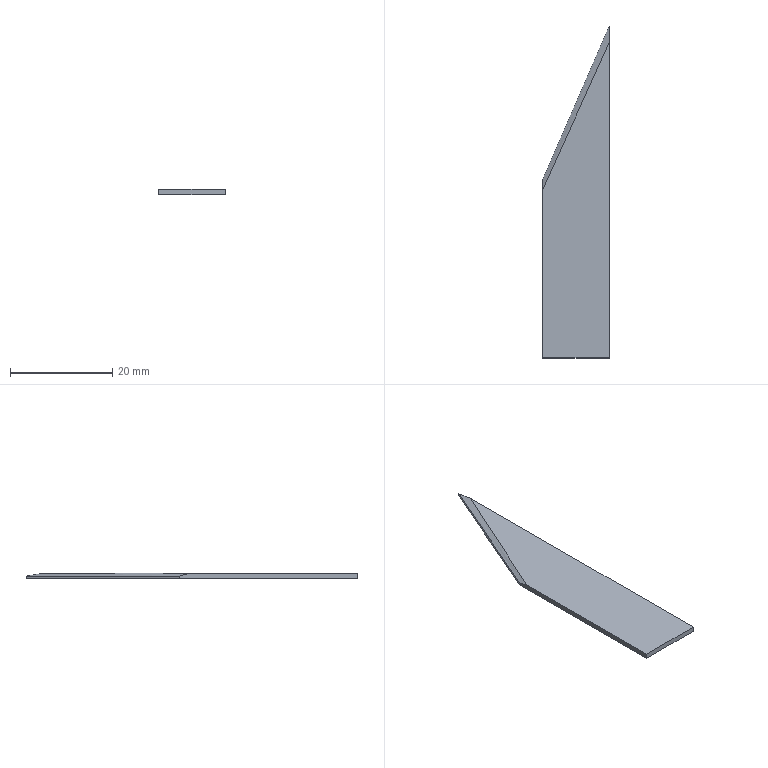Part | SolidWorks | features ICE 2, BlendCut 1, Extrusion 1 | 1 solid | 7 faces | box 13 x 65 x 1 mm | volume 641.482 mm3 | plane 6 | spline 1
STEP:
#1=CARTESIAN_POINT('',(6.5,35.,0.));
#2=VERTEX_POINT('',#1);
#3=CARTESIAN_POINT('',(6.5,35.,-0.5));
#4=VERTEX_POINT('',#3);
#5=CARTESIAN_POINT('',(6.5,35.,0.5));
#6=DIRECTION('',(0.,0.,-1.));
#7=VECTOR('',#6,1000.);
#8=LINE('',#5,#7);
#9=EDGE_CURVE('',#2,#4,#8,.T.);
#10=ORIENTED_EDGE('',*,*,#9,.F.);
#11=CARTESIAN_POINT('',(6.5,31.731,0.5));
#12=VERTEX_POINT('',#11);
#13=CARTESIAN_POINT('',(6.5,35.,0.));
#14=DIRECTION('',(0.,0.9885,-0.1512));
#15=VECTOR('',#14,1000.);
#16=LINE('',#13,#15);
#17=EDGE_CURVE('',#12,#2,#16,.T.);
#18=ORIENTED_EDGE('',*,*,#17,.F.);
#19=CARTESIAN_POINT('',(6.5,-30.,0.5));
#20=VERTEX_POINT('',#19);
#21=CARTESIAN_POINT('',(6.5,35.,0.5));
#22=DIRECTION('',(0.,-1.,0.));
#23=VECTOR('',#22,1000.);
#24=LINE('',#21,#23);
#25=EDGE_CURVE('',#12,#20,#24,.T.);
#26=ORIENTED_EDGE('',*,*,#25,.T.);
#27=CARTESIAN_POINT('',(6.5,-30.,-0.5));
#28=VERTEX_POINT('',#27);
#29=CARTESIAN_POINT('',(6.5,-30.,-0.5));
#30=DIRECTION('',(0.,0.,1.));
#31=VECTOR('',#30,1000.);
#32=LINE('',#29,#31);
#33=EDGE_CURVE('',#28,#20,#32,.T.);
#34=ORIENTED_EDGE('',*,*,#33,.F.);
#35=CARTESIAN_POINT('',(6.5,35.,-0.5));
#36=DIRECTION('',(0.,-1.,0.));
#37=VECTOR('',#36,1000.);
#38=LINE('',#35,#37);
#39=EDGE_CURVE('',#4,#28,#38,.T.);
#40=ORIENTED_EDGE('',*,*,#39,.F.);
#41=EDGE_LOOP('',(#10,#18,#26,#34,#40));
#42=FACE_OUTER_BOUND('',#41,.T.);
#43=CARTESIAN_POINT('',(6.5,35.,0.5));
#44=DIRECTION('',(-1.,0.,0.));
#45=DIRECTION('',(0.,0.,1.));
#46=AXIS2_PLACEMENT_3D('',#43,#44,#45);
#47=PLANE('',#46);
#48=ADVANCED_FACE('',(#42),#47,.F.);
#49=CARTESIAN_POINT('',(-6.5,5.,-0.5));
#50=VERTEX_POINT('',#49);
#51=CARTESIAN_POINT('',(-6.5,-30.,-0.5));
#52=VERTEX_POINT('',#51);
#53=CARTESIAN_POINT('',(-6.5,35.,-0.5));
#54=DIRECTION('',(0.,-1.,0.));
#55=VECTOR('',#54,1000.);
#56=LINE('',#53,#55);
#57=EDGE_CURVE('',#50,#52,#56,.T.);
#58=ORIENTED_EDGE('',*,*,#57,.F.);
#59=CARTESIAN_POINT('',(6.5,35.,-0.5));
#60=DIRECTION('',(0.3976,0.9176,0.));
#61=VECTOR('',#60,1000.);
#62=LINE('',#59,#61);
#63=EDGE_CURVE('',#50,#4,#62,.T.);
#64=ORIENTED_EDGE('',*,*,#63,.T.);
#65=ORIENTED_EDGE('',*,*,#39,.T.);
#66=CARTESIAN_POINT('',(-6.5,-30.,-0.5));
#67=DIRECTION('',(1.,0.,0.));
#68=VECTOR('',#67,1000.);
#69=LINE('',#66,#68);
#70=EDGE_CURVE('',#52,#28,#69,.T.);
#71=ORIENTED_EDGE('',*,*,#70,.F.);
#72=EDGE_LOOP('',(#58,#64,#65,#71));
#73=FACE_OUTER_BOUND('',#72,.T.);
#74=CARTESIAN_POINT('',(-6.5,35.,-0.5));
#75=DIRECTION('',(0.,0.,1.));
#76=DIRECTION('',(1.,0.,0.));
#77=AXIS2_PLACEMENT_3D('',#74,#75,#76);
#78=PLANE('',#77);
#79=ADVANCED_FACE('',(#73),#78,.F.);
#80=CARTESIAN_POINT('',(-6.5,3.028,0.5));
#81=VERTEX_POINT('',#80);
#82=CARTESIAN_POINT('',(-6.5,-30.,0.5));
#83=VERTEX_POINT('',#82);
#84=CARTESIAN_POINT('',(-6.5,35.,0.5));
#85=DIRECTION('',(0.,-1.,0.));
#86=VECTOR('',#85,1000.);
#87=LINE('',#84,#86);
#88=EDGE_CURVE('',#81,#83,#87,.T.);
#89=ORIENTED_EDGE('',*,*,#88,.F.);
#90=CARTESIAN_POINT('',(-6.5,5.,0.));
#91=VERTEX_POINT('',#90);
#92=CARTESIAN_POINT('',(-6.5,5.,0.));
#93=DIRECTION('',(0.,-0.9693,0.2457));
#94=VECTOR('',#93,1000.);
#95=LINE('',#92,#94);
#96=EDGE_CURVE('',#91,#81,#95,.T.);
#97=ORIENTED_EDGE('',*,*,#96,.F.);
#98=CARTESIAN_POINT('',(-6.5,5.,-0.5));
#99=DIRECTION('',(0.,0.,1.));
#100=VECTOR('',#99,1000.);
#101=LINE('',#98,#100);
#102=EDGE_CURVE('',#50,#91,#101,.T.);
#103=ORIENTED_EDGE('',*,*,#102,.F.);
#104=ORIENTED_EDGE('',*,*,#57,.T.);
#105=CARTESIAN_POINT('',(-6.5,-30.,0.5));
#106=DIRECTION('',(0.,0.,-1.));
#107=VECTOR('',#106,1000.);
#108=LINE('',#105,#107);
#109=EDGE_CURVE('',#83,#52,#108,.T.);
#110=ORIENTED_EDGE('',*,*,#109,.F.);
#111=EDGE_LOOP('',(#89,#97,#103,#104,#110));
#112=FACE_OUTER_BOUND('',#111,.T.);
#113=CARTESIAN_POINT('',(-6.5,35.,0.5));
#114=DIRECTION('',(1.,0.,0.));
#115=DIRECTION('',(0.,0.,-1.));
#116=AXIS2_PLACEMENT_3D('',#113,#114,#115);
#117=PLANE('',#116);
#118=ADVANCED_FACE('',(#112),#117,.F.);
#119=ORIENTED_EDGE('',*,*,#25,.F.);
#120=CARTESIAN_POINT('',(0.,17.379,0.5));
#121=DIRECTION('',(-0.4126,-0.9109,0.));
#122=VECTOR('',#121,1000.);
#123=LINE('',#120,#122);
#124=EDGE_CURVE('',#12,#81,#123,.T.);
#125=ORIENTED_EDGE('',*,*,#124,.T.);
#126=ORIENTED_EDGE('',*,*,#88,.T.);
#127=CARTESIAN_POINT('',(6.5,-30.,0.5));
#128=DIRECTION('',(-1.,0.,0.));
#129=VECTOR('',#128,1000.);
#130=LINE('',#127,#129);
#131=EDGE_CURVE('',#20,#83,#130,.T.);
#132=ORIENTED_EDGE('',*,*,#131,.F.);
#133=EDGE_LOOP('',(#119,#125,#126,#132));
#134=FACE_OUTER_BOUND('',#133,.T.);
#135=CARTESIAN_POINT('',(-6.5,35.,0.5));
#136=DIRECTION('',(0.,0.,-1.));
#137=DIRECTION('',(-1.,0.,0.));
#138=AXIS2_PLACEMENT_3D('',#135,#136,#137);
#139=PLANE('',#138);
#140=ADVANCED_FACE('',(#134),#139,.F.);
#141=ORIENTED_EDGE('',*,*,#102,.T.);
#142=CARTESIAN_POINT('',(0.,20.,0.));
#143=DIRECTION('',(0.3976,0.9176,0.));
#144=VECTOR('',#143,1000.);
#145=LINE('',#142,#144);
#146=EDGE_CURVE('',#91,#2,#145,.T.);
#147=ORIENTED_EDGE('',*,*,#146,.T.);
#148=ORIENTED_EDGE('',*,*,#9,.T.);
#149=ORIENTED_EDGE('',*,*,#63,.F.);
#150=EDGE_LOOP('',(#141,#147,#148,#149));
#151=FACE_OUTER_BOUND('',#150,.T.);
#152=CARTESIAN_POINT('',(6.5,35.,-0.5));
#153=DIRECTION('',(0.9176,-0.3976,0.));
#154=DIRECTION('',(0.3976,0.9176,0.));
#155=AXIS2_PLACEMENT_3D('',#152,#153,#154);
#156=PLANE('',#155);
#157=ADVANCED_FACE('',(#151),#156,.F.);
#158=ORIENTED_EDGE('',*,*,#17,.T.);
#159=ORIENTED_EDGE('',*,*,#146,.F.);
#160=ORIENTED_EDGE('',*,*,#96,.T.);
#161=ORIENTED_EDGE('',*,*,#124,.F.);
#162=EDGE_LOOP('',(#158,#159,#160,#161));
#163=FACE_OUTER_BOUND('',#162,.T.);
#164=CARTESIAN_POINT('',(6.5,35.,0.));
#165=CARTESIAN_POINT('',(-6.5,5.,0.));
#166=CARTESIAN_POINT('',(6.5,34.455,0.08333));
#167=CARTESIAN_POINT('',(-6.5,4.671,0.08333));
#168=CARTESIAN_POINT('',(6.5,33.91,0.1667));
#169=CARTESIAN_POINT('',(-6.5,4.343,0.1667));
#170=CARTESIAN_POINT('',(6.5,32.821,0.3333));
#171=CARTESIAN_POINT('',(-6.5,3.685,0.3333));
#172=CARTESIAN_POINT('',(6.5,32.276,0.4167));
#173=CARTESIAN_POINT('',(-6.5,3.356,0.4167));
#174=CARTESIAN_POINT('',(6.5,31.731,0.5));
#175=CARTESIAN_POINT('',(-6.5,3.028,0.5));
#176=B_SPLINE_SURFACE_WITH_KNOTS('',3,1,((#164,#165),(#166,#167),(#168,#169),(#170,#171),(#172,#173),(#174,#175)),.UNSPECIFIED.,.F.,.F.,.F.,(4,2,4),(2,2),(0.,0.5,1.),(0.,1.),.UNSPECIFIED.);
#177=ADVANCED_FACE('',(#163),#176,.F.);
#178=ORIENTED_EDGE('',*,*,#70,.T.);
#179=ORIENTED_EDGE('',*,*,#33,.T.);
#180=ORIENTED_EDGE('',*,*,#131,.T.);
#181=ORIENTED_EDGE('',*,*,#109,.T.);
#182=EDGE_LOOP('',(#178,#179,#180,#181));
#183=FACE_OUTER_BOUND('',#182,.T.);
#184=CARTESIAN_POINT('',(0.,-30.,0.));
#185=DIRECTION('',(0.,-1.,0.));
#186=DIRECTION('',(0.,0.,-1.));
#187=AXIS2_PLACEMENT_3D('',#184,#185,#186);
#188=PLANE('',#187);
#189=ADVANCED_FACE('',(#183),#188,.T.);
#190=CLOSED_SHELL('',(#48,#79,#118,#140,#157,#177,#189));
#191=MANIFOLD_SOLID_BREP('',#190);
#192=CARTESIAN_POINT('',(0.,0.,0.));
#193=DIRECTION('',(0.,0.,1.));
#194=DIRECTION('',(1.,0.,0.));
#195=AXIS2_PLACEMENT_3D('',#192,#193,#194);
#196=(LENGTH_UNIT()NAMED_UNIT(*)SI_UNIT(.MILLI.,.METRE.));
#197=UNCERTAINTY_MEASURE_WITH_UNIT(LENGTH_MEASURE(0.00001),#196,'','');
#198=(NAMED_UNIT(*)PLANE_ANGLE_UNIT()SI_UNIT($,.RADIAN.));
#199=(NAMED_UNIT(*)SI_UNIT($,.STERADIAN.)SOLID_ANGLE_UNIT());
#200=(GEOMETRIC_REPRESENTATION_CONTEXT(3)GLOBAL_UNCERTAINTY_ASSIGNED_CONTEXT((#197))GLOBAL_UNIT_ASSIGNED_CONTEXT((#196,#198,#199))REPRESENTATION_CONTEXT('',''));
#201=ADVANCED_BREP_SHAPE_REPRESENTATION('',(#191,#195),#200);